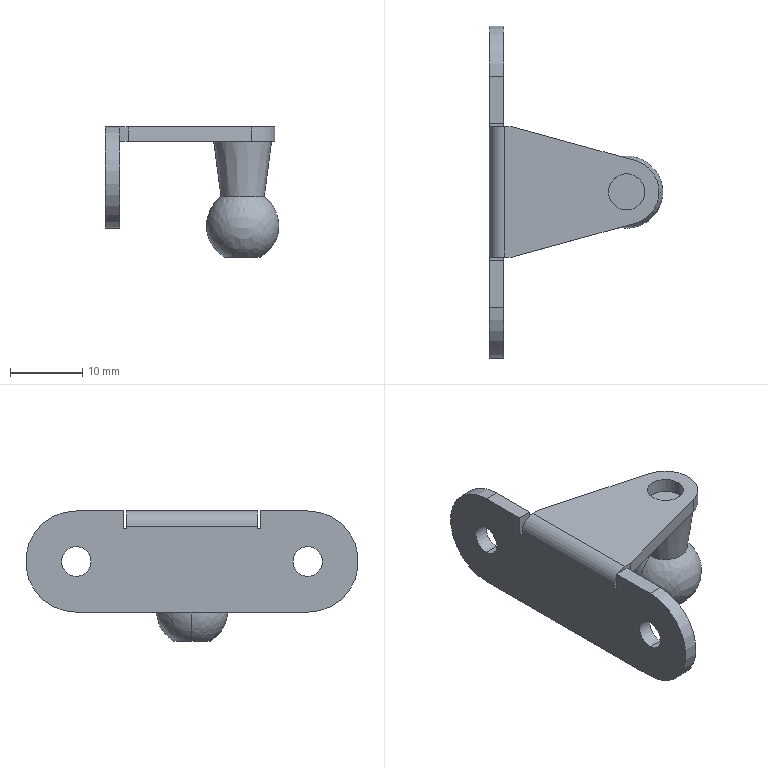Part | STEP file | damper support B | 1 solid | 32 faces | box 24 x 46 x 18 mm | volume 2428 mm3 | plane 17 | cylinder 11 | spline 2 | cone 2 | commonest cylinder face diameters 4.1 x4 5 x2 14 x2 0.2 x1 4.2 x1 9 x1